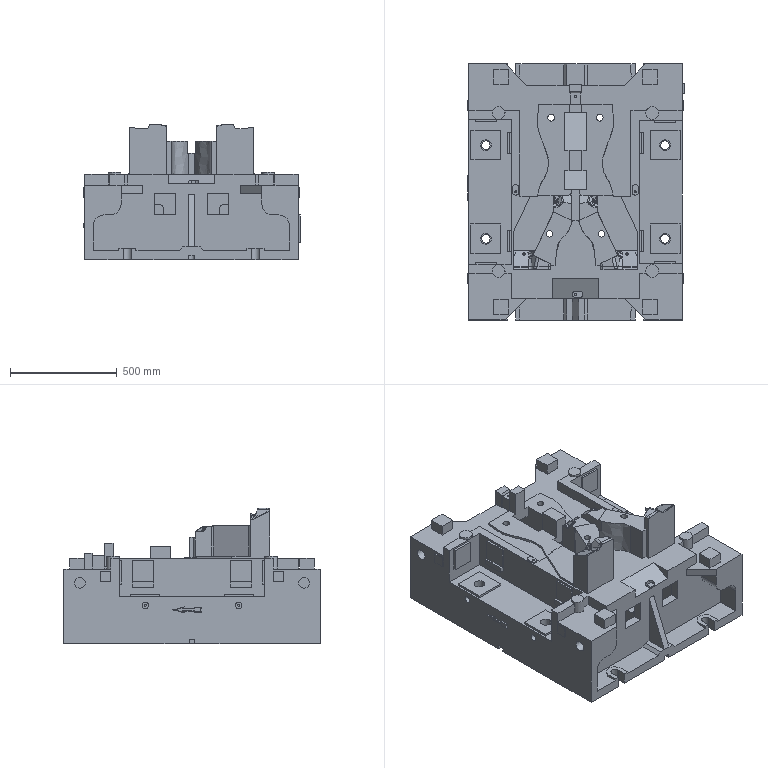Part | NX | features solid 2 | 1 solid | 754 faces | box 1015 x 1200 x 635.361 mm | volume 198285947 mm3 | plane 517 | spline 136 | cylinder 101 | commonest cylinder face diameters 40 x44 30 x14 50 x9 10 x8 100 x8 20 x6